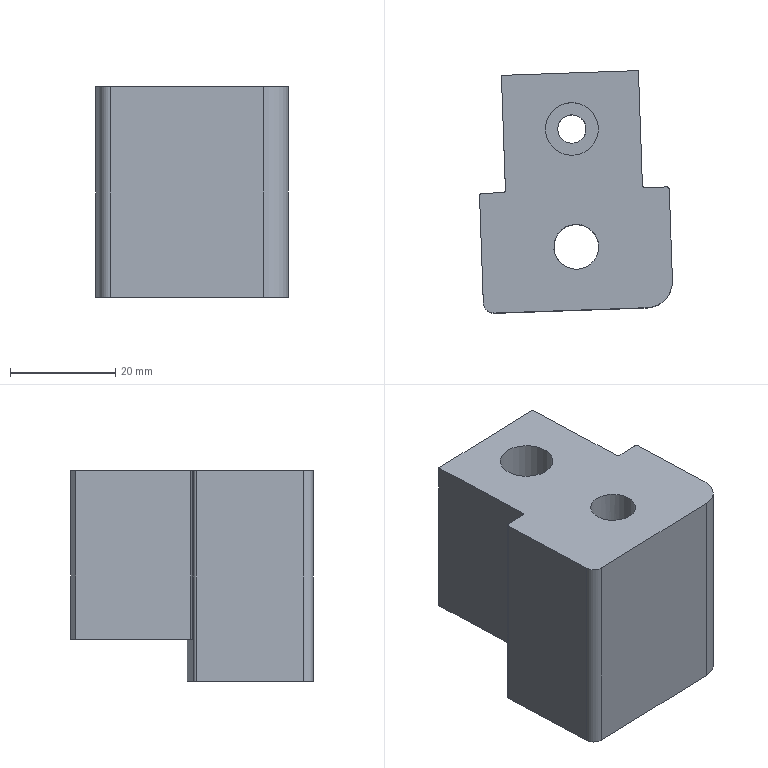Part | NX | features PS-24 2 | 1 solid | 22 faces | box 36.584 x 45.984 x 40 mm | volume 45410 mm3 | plane 12 | cylinder 10 | commonest cylinder face diameters 1 x4 10 x2 4 x1 5.4 x1 8.506 x1 14.5 x1
STEP:
#1=CARTESIAN_POINT('',(3172.903,-799.38,868.716));
#2=VERTEX_POINT('',#1);
#3=CARTESIAN_POINT('',(3198.887,-798.472,868.716));
#4=VERTEX_POINT('',#3);
#5=CARTESIAN_POINT('',(3185.895,-798.926,868.716));
#6=DIRECTION('',(0.9994,0.0349,0.));
#7=VECTOR('',#6,1000.);
#8=LINE('',#5,#7);
#9=EDGE_CURVE('',#2,#4,#8,.T.);
#10=ORIENTED_EDGE('',*,*,#9,.T.);
#11=CARTESIAN_POINT('',(3199.646,-820.196,868.716));
#12=VERTEX_POINT('',#11);
#13=CARTESIAN_POINT('',(3198.921,-799.44,868.716));
#14=DIRECTION('',(0.0349,-0.9994,0.));
#15=VECTOR('',#14,1000.);
#16=LINE('',#13,#15);
#17=EDGE_CURVE('',#4,#12,#16,.T.);
#18=ORIENTED_EDGE('',*,*,#17,.T.);
#19=CARTESIAN_POINT('',(3200.163,-820.678,868.716));
#20=VERTEX_POINT('',#19);
#21=CARTESIAN_POINT('',(3200.145,-820.179,868.716));
#22=DIRECTION('',(0.,0.,1.));
#23=DIRECTION('',(-1.,0.,0.));
#24=AXIS2_PLACEMENT_3D('',#21,#22,#23);
#25=CIRCLE('',#24,0.5);
#26=EDGE_CURVE('',#20,#12,#25,.F.);
#27=ORIENTED_EDGE('',*,*,#26,.F.);
#28=CARTESIAN_POINT('',(3173.179,-821.621,868.716));
#29=VERTEX_POINT('',#28);
#30=CARTESIAN_POINT('',(3186.671,-821.149,868.716));
#31=DIRECTION('',(0.9994,0.0349,0.));
#32=VECTOR('',#31,1000.);
#33=LINE('',#30,#32);
#34=EDGE_CURVE('',#29,#20,#33,.T.);
#35=ORIENTED_EDGE('',*,*,#34,.F.);
#36=CARTESIAN_POINT('',(3173.662,-821.103,868.716));
#37=VERTEX_POINT('',#36);
#38=CARTESIAN_POINT('',(3173.162,-821.121,868.716));
#39=DIRECTION('',(0.,0.,1.));
#40=DIRECTION('',(-1.,0.,0.));
#41=AXIS2_PLACEMENT_3D('',#38,#39,#40);
#42=CIRCLE('',#41,0.5);
#43=EDGE_CURVE('',#37,#29,#42,.F.);
#44=ORIENTED_EDGE('',*,*,#43,.F.);
#45=CARTESIAN_POINT('',(3172.937,-800.347,868.716));
#46=DIRECTION('',(-0.0349,0.9994,0.));
#47=VECTOR('',#46,1000.);
#48=LINE('',#45,#47);
#49=EDGE_CURVE('',#2,#37,#48,.F.);
#50=ORIENTED_EDGE('',*,*,#49,.F.);
#51=EDGE_LOOP('',(#10,#18,#27,#35,#44,#50));
#52=FACE_BOUND('',#51,.T.);
#53=CARTESIAN_POINT('',(3183.566,-809.538,868.716));
#54=VERTEX_POINT('',#53);
#55=CARTESIAN_POINT('',(3186.266,-809.538,868.716));
#56=DIRECTION('',(0.,0.,1.));
#57=DIRECTION('',(-1.,0.,0.));
#58=AXIS2_PLACEMENT_3D('',#55,#56,#57);
#59=CIRCLE('',#58,2.7);
#60=EDGE_CURVE('',#54,#54,#59,.F.);
#61=ORIENTED_EDGE('',*,*,#60,.F.);
#62=EDGE_LOOP('',(#61));
#63=FACE_BOUND('',#62,.T.);
#64=CARTESIAN_POINT('',(3186.266,-809.538,868.716));
#65=DIRECTION('',(0.,0.,-1.));
#66=DIRECTION('',(-0.0349,0.9994,0.));
#67=AXIS2_PLACEMENT_3D('',#64,#65,#66);
#68=PLANE('',#67);
#69=ADVANCED_FACE('',(#52,#63),#68,.T.);
#70=CARTESIAN_POINT('',(3186.266,-804.538,900.716));
#71=VERTEX_POINT('',#70);
#72=CARTESIAN_POINT('',(3186.266,-809.538,900.716));
#73=DIRECTION('',(0.,0.,-1.));
#74=DIRECTION('',(0.,1.,0.));
#75=AXIS2_PLACEMENT_3D('',#72,#73,#74);
#76=CIRCLE('',#75,5.);
#77=EDGE_CURVE('',#71,#71,#76,.T.);
#78=ORIENTED_EDGE('',*,*,#77,.T.);
#79=EDGE_LOOP('',(#78));
#80=FACE_BOUND('',#79,.T.);
#81=CARTESIAN_POINT('',(3172.903,-799.38,900.716));
#82=VERTEX_POINT('',#81);
#83=CARTESIAN_POINT('',(3173.662,-821.103,900.716));
#84=VERTEX_POINT('',#83);
#85=CARTESIAN_POINT('',(3172.937,-800.347,900.716));
#86=DIRECTION('',(0.0349,-0.9994,0.));
#87=VECTOR('',#86,1000.);
#88=LINE('',#85,#87);
#89=EDGE_CURVE('',#82,#84,#88,.T.);
#90=ORIENTED_EDGE('',*,*,#89,.T.);
#91=CARTESIAN_POINT('',(3173.179,-821.621,900.716));
#92=VERTEX_POINT('',#91);
#93=CARTESIAN_POINT('',(3173.162,-821.121,900.716));
#94=DIRECTION('',(0.,0.,-1.));
#95=DIRECTION('',(0.,1.,0.));
#96=AXIS2_PLACEMENT_3D('',#93,#94,#95);
#97=CIRCLE('',#96,0.5);
#98=EDGE_CURVE('',#92,#84,#97,.F.);
#99=ORIENTED_EDGE('',*,*,#98,.F.);
#100=CARTESIAN_POINT('',(3169.242,-821.758,900.716));
#101=VERTEX_POINT('',#100);
#102=CARTESIAN_POINT('',(3027.832,-826.696,900.716));
#103=DIRECTION('',(-0.9994,-0.0349,0.));
#104=VECTOR('',#103,1000.);
#105=LINE('',#102,#104);
#106=EDGE_CURVE('',#101,#92,#105,.F.);
#107=ORIENTED_EDGE('',*,*,#106,.F.);
#108=CARTESIAN_POINT('',(3168.76,-822.275,900.716));
#109=VERTEX_POINT('',#108);
#110=CARTESIAN_POINT('',(3169.26,-822.258,900.716));
#111=DIRECTION('',(0.,0.,-1.));
#112=DIRECTION('',(0.,1.,0.));
#113=AXIS2_PLACEMENT_3D('',#110,#111,#112);
#114=CIRCLE('',#113,0.5);
#115=EDGE_CURVE('',#109,#101,#114,.T.);
#116=ORIENTED_EDGE('',*,*,#115,.F.);
#117=CARTESIAN_POINT('',(3169.467,-842.526,900.716));
#118=VERTEX_POINT('',#117);
#119=CARTESIAN_POINT('',(3166.834,-767.126,900.716));
#120=DIRECTION('',(-0.0349,0.9994,0.));
#121=VECTOR('',#120,1000.);
#122=LINE('',#119,#121);
#123=EDGE_CURVE('',#109,#118,#122,.F.);
#124=ORIENTED_EDGE('',*,*,#123,.T.);
#125=CARTESIAN_POINT('',(3171.536,-844.455,900.716));
#126=VERTEX_POINT('',#125);
#127=CARTESIAN_POINT('',(3171.466,-842.456,900.716));
#128=DIRECTION('',(0.,0.,-1.));
#129=DIRECTION('',(0.,1.,0.));
#130=AXIS2_PLACEMENT_3D('',#127,#128,#129);
#131=CIRCLE('',#130,2.);
#132=EDGE_CURVE('',#118,#126,#131,.F.);
#133=ORIENTED_EDGE('',*,*,#132,.T.);
#134=CARTESIAN_POINT('',(3200.518,-843.443,900.716));
#135=VERTEX_POINT('',#134);
#136=CARTESIAN_POINT('',(3158.544,-844.908,900.716));
#137=DIRECTION('',(-0.9994,-0.0349,0.));
#138=VECTOR('',#137,1000.);
#139=LINE('',#136,#138);
#140=EDGE_CURVE('',#135,#126,#139,.T.);
#141=ORIENTED_EDGE('',*,*,#140,.F.);
#142=CARTESIAN_POINT('',(3205.34,-838.271,900.716));
#143=VERTEX_POINT('',#142);
#144=CARTESIAN_POINT('',(3200.343,-838.446,900.716));
#145=DIRECTION('',(0.,0.,-1.));
#146=DIRECTION('',(0.,1.,0.));
#147=AXIS2_PLACEMENT_3D('',#144,#145,#146);
#148=CIRCLE('',#147,5.);
#149=EDGE_CURVE('',#135,#143,#148,.F.);
#150=ORIENTED_EDGE('',*,*,#149,.T.);
#151=CARTESIAN_POINT('',(3204.738,-821.019,900.716));
#152=VERTEX_POINT('',#151);
#153=CARTESIAN_POINT('',(3202.812,-765.869,900.716));
#154=DIRECTION('',(-0.0349,0.9994,0.));
#155=VECTOR('',#154,1000.);
#156=LINE('',#153,#155);
#157=EDGE_CURVE('',#152,#143,#156,.F.);
#158=ORIENTED_EDGE('',*,*,#157,.F.);
#159=CARTESIAN_POINT('',(3204.221,-820.537,900.716));
#160=VERTEX_POINT('',#159);
#161=CARTESIAN_POINT('',(3204.238,-821.036,900.716));
#162=DIRECTION('',(0.,0.,-1.));
#163=DIRECTION('',(0.,1.,0.));
#164=AXIS2_PLACEMENT_3D('',#161,#162,#163);
#165=CIRCLE('',#164,0.5);
#166=EDGE_CURVE('',#160,#152,#165,.T.);
#167=ORIENTED_EDGE('',*,*,#166,.F.);
#168=CARTESIAN_POINT('',(3200.163,-820.678,900.716));
#169=VERTEX_POINT('',#168);
#170=CARTESIAN_POINT('',(3027.832,-826.696,900.716));
#171=DIRECTION('',(-0.9994,-0.0349,0.));
#172=VECTOR('',#171,1000.);
#173=LINE('',#170,#172);
#174=EDGE_CURVE('',#169,#160,#173,.F.);
#175=ORIENTED_EDGE('',*,*,#174,.F.);
#176=CARTESIAN_POINT('',(3199.646,-820.196,900.716));
#177=VERTEX_POINT('',#176);
#178=CARTESIAN_POINT('',(3200.145,-820.179,900.716));
#179=DIRECTION('',(0.,0.,-1.));
#180=DIRECTION('',(0.,1.,0.));
#181=AXIS2_PLACEMENT_3D('',#178,#179,#180);
#182=CIRCLE('',#181,0.5);
#183=EDGE_CURVE('',#177,#169,#182,.F.);
#184=ORIENTED_EDGE('',*,*,#183,.F.);
#185=CARTESIAN_POINT('',(3198.887,-798.472,900.716));
#186=VERTEX_POINT('',#185);
#187=CARTESIAN_POINT('',(3198.921,-799.44,900.716));
#188=DIRECTION('',(-0.0349,0.9994,0.));
#189=VECTOR('',#188,1000.);
#190=LINE('',#187,#189);
#191=EDGE_CURVE('',#186,#177,#190,.F.);
#192=ORIENTED_EDGE('',*,*,#191,.F.);
#193=CARTESIAN_POINT('',(3027.056,-804.472,900.716));
#194=DIRECTION('',(-0.9994,-0.0349,0.));
#195=VECTOR('',#194,1000.);
#196=LINE('',#193,#195);
#197=EDGE_CURVE('',#82,#186,#196,.F.);
#198=ORIENTED_EDGE('',*,*,#197,.F.);
#199=EDGE_LOOP('',(#90,#99,#107,#116,#124,#133,#141,#150,#158,#167,#175,#184,#192,#198));
#200=FACE_BOUND('',#199,.T.);
#201=CARTESIAN_POINT('',(3187.107,-827.651,900.716));
#202=VERTEX_POINT('',#201);
#203=CARTESIAN_POINT('',(3187.107,-831.904,900.716));
#204=DIRECTION('',(0.,0.,-1.));
#205=DIRECTION('',(0.,1.,0.));
#206=AXIS2_PLACEMENT_3D('',#203,#204,#205);
#207=CIRCLE('',#206,4.253);
#208=EDGE_CURVE('',#202,#202,#207,.T.);
#209=ORIENTED_EDGE('',*,*,#208,.T.);
#210=EDGE_LOOP('',(#209));
#211=FACE_BOUND('',#210,.T.);
#212=CARTESIAN_POINT('',(3025.924,-772.046,900.716));
#213=DIRECTION('',(0.,0.,1.));
#214=DIRECTION('',(0.9976,0.06975,0.));
#215=AXIS2_PLACEMENT_3D('',#212,#213,#214);
#216=PLANE('',#215);
#217=ADVANCED_FACE('',(#80,#200,#211),#216,.T.);
#218=ORIENTED_EDGE('',*,*,#17,.F.);
#219=CARTESIAN_POINT('',(3198.887,-798.472,880.716));
#220=DIRECTION('',(0.,0.,-1.));
#221=VECTOR('',#220,1000.);
#222=LINE('',#219,#221);
#223=EDGE_CURVE('',#186,#4,#222,.T.);
#224=ORIENTED_EDGE('',*,*,#223,.F.);
#225=ORIENTED_EDGE('',*,*,#191,.T.);
#226=CARTESIAN_POINT('',(3199.646,-820.196,830.716));
#227=DIRECTION('',(0.,0.,1.));
#228=VECTOR('',#227,1000.);
#229=LINE('',#226,#228);
#230=EDGE_CURVE('',#12,#177,#229,.T.);
#231=ORIENTED_EDGE('',*,*,#230,.F.);
#232=EDGE_LOOP('',(#218,#224,#225,#231));
#233=FACE_BOUND('',#232,.T.);
#234=CARTESIAN_POINT('',(3198.921,-799.44,830.716));
#235=DIRECTION('',(0.9994,0.0349,0.));
#236=DIRECTION('',(0.0349,-0.9994,0.));
#237=AXIS2_PLACEMENT_3D('',#234,#235,#236);
#238=PLANE('',#237);
#239=ADVANCED_FACE('',(#233),#238,.T.);
#240=ORIENTED_EDGE('',*,*,#49,.T.);
#241=CARTESIAN_POINT('',(3173.662,-821.103,863.216));
#242=DIRECTION('',(0.,0.,1.));
#243=VECTOR('',#242,1000.);
#244=LINE('',#241,#243);
#245=EDGE_CURVE('',#84,#37,#244,.F.);
#246=ORIENTED_EDGE('',*,*,#245,.F.);
#247=ORIENTED_EDGE('',*,*,#89,.F.);
#248=CARTESIAN_POINT('',(3172.903,-799.38,830.716));
#249=DIRECTION('',(0.,0.,-1.));
#250=VECTOR('',#249,1000.);
#251=LINE('',#248,#250);
#252=EDGE_CURVE('',#82,#2,#251,.T.);
#253=ORIENTED_EDGE('',*,*,#252,.T.);
#254=EDGE_LOOP('',(#240,#246,#247,#253));
#255=FACE_BOUND('',#254,.T.);
#256=CARTESIAN_POINT('',(3172.937,-800.347,830.716));
#257=DIRECTION('',(-0.9994,-0.0349,0.));
#258=DIRECTION('',(-0.0349,0.9994,0.));
#259=AXIS2_PLACEMENT_3D('',#256,#257,#258);
#260=PLANE('',#259);
#261=ADVANCED_FACE('',(#255),#260,.T.);
#262=CARTESIAN_POINT('',(3186.266,-814.538,890.716));
#263=VERTEX_POINT('',#262);
#264=CARTESIAN_POINT('',(3186.266,-809.538,890.716));
#265=DIRECTION('',(0.,0.,1.));
#266=DIRECTION('',(0.,-1.,0.));
#267=AXIS2_PLACEMENT_3D('',#264,#265,#266);
#268=CIRCLE('',#267,5.);
#269=EDGE_CURVE('',#263,#263,#268,.F.);
#270=ORIENTED_EDGE('',*,*,#269,.T.);
#271=EDGE_LOOP('',(#270));
#272=FACE_BOUND('',#271,.T.);
#273=ORIENTED_EDGE('',*,*,#77,.F.);
#274=EDGE_LOOP('',(#273));
#275=FACE_BOUND('',#274,.T.);
#276=CARTESIAN_POINT('',(3186.266,-809.538,935.716));
#277=DIRECTION('',(0.,0.,-1.));
#278=DIRECTION('',(0.9976,0.06975,0.));
#279=AXIS2_PLACEMENT_3D('',#276,#277,#278);
#280=CYLINDRICAL_SURFACE('',#279,5.);
#281=ADVANCED_FACE('',(#272,#275),#280,.F.);
#282=ORIENTED_EDGE('',*,*,#60,.T.);
#283=EDGE_LOOP('',(#282));
#284=FACE_BOUND('',#283,.T.);
#285=CARTESIAN_POINT('',(3186.266,-812.238,890.716));
#286=VERTEX_POINT('',#285);
#287=CARTESIAN_POINT('',(3186.266,-809.538,890.716));
#288=DIRECTION('',(0.,0.,1.));
#289=DIRECTION('',(0.,-1.,0.));
#290=AXIS2_PLACEMENT_3D('',#287,#288,#289);
#291=CIRCLE('',#290,2.7);
#292=EDGE_CURVE('',#286,#286,#291,.T.);
#293=ORIENTED_EDGE('',*,*,#292,.T.);
#294=EDGE_LOOP('',(#293));
#295=FACE_BOUND('',#294,.T.);
#296=CARTESIAN_POINT('',(3186.266,-809.538,872.716));
#297=DIRECTION('',(0.,0.,-1.));
#298=DIRECTION('',(0.9976,0.06975,0.));
#299=AXIS2_PLACEMENT_3D('',#296,#297,#298);
#300=CYLINDRICAL_SURFACE('',#299,2.7);
#301=ADVANCED_FACE('',(#284,#295),#300,.F.);
#302=ORIENTED_EDGE('',*,*,#292,.F.);
#303=EDGE_LOOP('',(#302));
#304=FACE_BOUND('',#303,.T.);
#305=ORIENTED_EDGE('',*,*,#269,.F.);
#306=EDGE_LOOP('',(#305));
#307=FACE_BOUND('',#306,.T.);
#308=CARTESIAN_POINT('',(3186.266,-809.538,890.716));
#309=DIRECTION('',(0.,0.,-1.));
#310=DIRECTION('',(-0.9976,-0.06975,0.));
#311=AXIS2_PLACEMENT_3D('',#308,#309,#310);
#312=PLANE('',#311);
#313=ADVANCED_FACE('',(#304,#307),#312,.F.);
#314=ORIENTED_EDGE('',*,*,#183,.T.);
#315=CARTESIAN_POINT('',(3200.163,-820.678,863.216));
#316=DIRECTION('',(0.,0.,1.));
#317=VECTOR('',#316,1000.);
#318=LINE('',#315,#317);
#319=EDGE_CURVE('',#169,#20,#318,.F.);
#320=ORIENTED_EDGE('',*,*,#319,.T.);
#321=ORIENTED_EDGE('',*,*,#26,.T.);
#322=ORIENTED_EDGE('',*,*,#230,.T.);
#323=EDGE_LOOP('',(#314,#320,#321,#322));
#324=FACE_BOUND('',#323,.T.);
#325=CARTESIAN_POINT('',(3200.145,-820.179,830.716));
#326=DIRECTION('',(0.,0.,1.));
#327=DIRECTION('',(0.,1.,0.));
#328=AXIS2_PLACEMENT_3D('',#325,#326,#327);
#329=CYLINDRICAL_SURFACE('',#328,0.5);
#330=ADVANCED_FACE('',(#324),#329,.F.);
#331=ORIENTED_EDGE('',*,*,#98,.T.);
#332=ORIENTED_EDGE('',*,*,#245,.T.);
#333=ORIENTED_EDGE('',*,*,#43,.T.);
#334=CARTESIAN_POINT('',(3173.179,-821.621,863.216));
#335=DIRECTION('',(0.,0.,-1.));
#336=VECTOR('',#335,1000.);
#337=LINE('',#334,#336);
#338=EDGE_CURVE('',#29,#92,#337,.F.);
#339=ORIENTED_EDGE('',*,*,#338,.T.);
#340=EDGE_LOOP('',(#331,#332,#333,#339));
#341=FACE_BOUND('',#340,.T.);
#342=CARTESIAN_POINT('',(3173.162,-821.121,863.216));
#343=DIRECTION('',(0.,0.,1.));
#344=DIRECTION('',(0.,1.,0.));
#345=AXIS2_PLACEMENT_3D('',#342,#343,#344);
#346=CYLINDRICAL_SURFACE('',#345,0.5);
#347=ADVANCED_FACE('',(#341),#346,.F.);
#348=ORIENTED_EDGE('',*,*,#34,.T.);
#349=ORIENTED_EDGE('',*,*,#319,.F.);
#350=ORIENTED_EDGE('',*,*,#174,.T.);
#351=CARTESIAN_POINT('',(3204.221,-820.537,860.716));
#352=VERTEX_POINT('',#351);
#353=CARTESIAN_POINT('',(3204.221,-820.537,890.716));
#354=DIRECTION('',(0.,0.,1.));
#355=VECTOR('',#354,1000.);
#356=LINE('',#353,#355);
#357=EDGE_CURVE('',#352,#160,#356,.T.);
#358=ORIENTED_EDGE('',*,*,#357,.F.);
#359=CARTESIAN_POINT('',(3169.242,-821.758,860.716));
#360=VERTEX_POINT('',#359);
#361=CARTESIAN_POINT('',(2864.273,-832.407,860.716));
#362=DIRECTION('',(0.9994,0.0349,0.));
#363=VECTOR('',#362,1000.);
#364=LINE('',#361,#363);
#365=EDGE_CURVE('',#352,#360,#364,.F.);
#366=ORIENTED_EDGE('',*,*,#365,.T.);
#367=CARTESIAN_POINT('',(3169.242,-821.758,863.216));
#368=DIRECTION('',(0.,0.,1.));
#369=VECTOR('',#368,1000.);
#370=LINE('',#367,#369);
#371=EDGE_CURVE('',#101,#360,#370,.F.);
#372=ORIENTED_EDGE('',*,*,#371,.F.);
#373=ORIENTED_EDGE('',*,*,#106,.T.);
#374=ORIENTED_EDGE('',*,*,#338,.F.);
#375=EDGE_LOOP('',(#348,#349,#350,#358,#366,#372,#373,#374));
#376=FACE_BOUND('',#375,.T.);
#377=CARTESIAN_POINT('',(3183.542,-821.259,863.216));
#378=DIRECTION('',(0.0349,-0.9994,0.));
#379=DIRECTION('',(-0.9994,-0.0349,0.));
#380=AXIS2_PLACEMENT_3D('',#377,#378,#379);
#381=PLANE('',#380);
#382=ADVANCED_FACE('',(#376),#381,.F.);
#383=CARTESIAN_POINT('',(3191.35,-831.607,879.716));
#384=VERTEX_POINT('',#383);
#385=CARTESIAN_POINT('',(3187.107,-831.904,879.716));
#386=DIRECTION('',(0.,0.,1.));
#387=DIRECTION('',(0.9976,0.06975,0.));
#388=AXIS2_PLACEMENT_3D('',#385,#386,#387);
#389=CIRCLE('',#388,4.253);
#390=EDGE_CURVE('',#384,#384,#389,.T.);
#391=ORIENTED_EDGE('',*,*,#390,.T.);
#392=EDGE_LOOP('',(#391));
#393=FACE_BOUND('',#392,.T.);
#394=CARTESIAN_POINT('',(3194.339,-831.398,879.716));
#395=VERTEX_POINT('',#394);
#396=CARTESIAN_POINT('',(3187.107,-831.904,879.716));
#397=DIRECTION('',(0.,0.,-1.));
#398=DIRECTION('',(0.9976,0.06975,0.));
#399=AXIS2_PLACEMENT_3D('',#396,#397,#398);
#400=CIRCLE('',#399,7.25);
#401=EDGE_CURVE('',#395,#395,#400,.F.);
#402=ORIENTED_EDGE('',*,*,#401,.F.);
#403=EDGE_LOOP('',(#402));
#404=FACE_BOUND('',#403,.T.);
#405=CARTESIAN_POINT('',(3187.107,-831.904,879.716));
#406=DIRECTION('',(0.,0.,1.));
#407=DIRECTION('',(0.9976,0.06975,0.));
#408=AXIS2_PLACEMENT_3D('',#405,#406,#407);
#409=PLANE('',#408);
#410=ADVANCED_FACE('',(#393,#404),#409,.F.);
#411=ORIENTED_EDGE('',*,*,#390,.F.);
#412=EDGE_LOOP('',(#411));
#413=FACE_BOUND('',#412,.T.);
#414=ORIENTED_EDGE('',*,*,#208,.F.);
#415=EDGE_LOOP('',(#414));
#416=FACE_BOUND('',#415,.T.);
#417=CARTESIAN_POINT('',(3187.107,-831.904,868.716));
#418=DIRECTION('',(0.,0.,1.));
#419=DIRECTION('',(0.9976,0.06975,0.));
#420=AXIS2_PLACEMENT_3D('',#417,#418,#419);
#421=CYLINDRICAL_SURFACE('',#420,4.253);
#422=ADVANCED_FACE('',(#413,#416),#421,.F.);
#423=CARTESIAN_POINT('',(3168.76,-822.275,860.716));
#424=VERTEX_POINT('',#423);
#425=CARTESIAN_POINT('',(3169.26,-822.258,860.716));
#426=DIRECTION('',(0.,0.,1.));
#427=DIRECTION('',(1.,0.,0.));
#428=AXIS2_PLACEMENT_3D('',#425,#426,#427);
#429=CIRCLE('',#428,0.5);
#430=EDGE_CURVE('',#360,#424,#429,.T.);
#431=ORIENTED_EDGE('',*,*,#430,.T.);
#432=CARTESIAN_POINT('',(3168.76,-822.275,890.716));
#433=DIRECTION('',(0.,0.,1.));
#434=VECTOR('',#433,1000.);
#435=LINE('',#432,#434);
#436=EDGE_CURVE('',#424,#109,#435,.T.);
#437=ORIENTED_EDGE('',*,*,#436,.T.);
#438=ORIENTED_EDGE('',*,*,#115,.T.);
#439=ORIENTED_EDGE('',*,*,#371,.T.);
#440=EDGE_LOOP('',(#431,#437,#438,#439));
#441=FACE_BOUND('',#440,.T.);
#442=CARTESIAN_POINT('',(3169.26,-822.258,890.716));
#443=DIRECTION('',(0.,0.,1.));
#444=DIRECTION('',(1.,0.,0.));
#445=AXIS2_PLACEMENT_3D('',#442,#443,#444);
#446=CYLINDRICAL_SURFACE('',#445,0.5);
#447=ADVANCED_FACE('',(#441),#446,.T.);
#448=CARTESIAN_POINT('',(3169.467,-842.526,860.716));
#449=VERTEX_POINT('',#448);
#450=CARTESIAN_POINT('',(3174.564,-988.491,860.716));
#451=DIRECTION('',(-0.0349,0.9994,0.));
#452=VECTOR('',#451,1000.);
#453=LINE('',#450,#452);
#454=EDGE_CURVE('',#424,#449,#453,.F.);
#455=ORIENTED_EDGE('',*,*,#454,.T.);
#456=CARTESIAN_POINT('',(3169.467,-842.526,890.716));
#457=DIRECTION('',(0.,0.,1.));
#458=VECTOR('',#457,1000.);
#459=LINE('',#456,#458);
#460=EDGE_CURVE('',#449,#118,#459,.T.);
#461=ORIENTED_EDGE('',*,*,#460,.T.);
#462=ORIENTED_EDGE('',*,*,#123,.F.);
#463=ORIENTED_EDGE('',*,*,#436,.F.);
#464=EDGE_LOOP('',(#455,#461,#462,#463));
#465=FACE_BOUND('',#464,.T.);
#466=CARTESIAN_POINT('',(3168.523,-815.501,890.716));
#467=DIRECTION('',(0.9994,0.0349,0.));
#468=DIRECTION('',(-0.0349,0.9994,0.));
#469=AXIS2_PLACEMENT_3D('',#466,#467,#468);
#470=PLANE('',#469);
#471=ADVANCED_FACE('',(#465),#470,.F.);
#472=ORIENTED_EDGE('',*,*,#132,.F.);
#473=ORIENTED_EDGE('',*,*,#460,.F.);
#474=CARTESIAN_POINT('',(3171.536,-844.455,860.716));
#475=VERTEX_POINT('',#474);
#476=CARTESIAN_POINT('',(3171.466,-842.456,860.716));
#477=DIRECTION('',(0.,0.,1.));
#478=DIRECTION('',(1.,0.,0.));
#479=AXIS2_PLACEMENT_3D('',#476,#477,#478);
#480=CIRCLE('',#479,2.);
#481=EDGE_CURVE('',#475,#449,#480,.F.);
#482=ORIENTED_EDGE('',*,*,#481,.F.);
#483=CARTESIAN_POINT('',(3171.536,-844.455,860.716));
#484=DIRECTION('',(0.,0.,-1.));
#485=VECTOR('',#484,1000.);
#486=LINE('',#483,#485);
#487=EDGE_CURVE('',#126,#475,#486,.T.);
#488=ORIENTED_EDGE('',*,*,#487,.F.);
#489=EDGE_LOOP('',(#472,#473,#482,#488));
#490=FACE_BOUND('',#489,.T.);
#491=CARTESIAN_POINT('',(3171.466,-842.456,935.716));
#492=DIRECTION('',(0.,0.,-1.));
#493=DIRECTION('',(-0.9976,-0.06975,0.));
#494=AXIS2_PLACEMENT_3D('',#491,#492,#493);
#495=CYLINDRICAL_SURFACE('',#494,2.);
#496=ADVANCED_FACE('',(#490),#495,.T.);
#497=CARTESIAN_POINT('',(3200.518,-843.443,860.716));
#498=VERTEX_POINT('',#497);
#499=CARTESIAN_POINT('',(3158.544,-844.908,860.716));
#500=DIRECTION('',(0.9994,0.0349,0.));
#501=VECTOR('',#500,1000.);
#502=LINE('',#499,#501);
#503=EDGE_CURVE('',#475,#498,#502,.T.);
#504=ORIENTED_EDGE('',*,*,#503,.T.);
#505=CARTESIAN_POINT('',(3200.518,-843.443,935.716));
#506=DIRECTION('',(0.,0.,-1.));
#507=VECTOR('',#506,1000.);
#508=LINE('',#505,#507);
#509=EDGE_CURVE('',#498,#135,#508,.F.);
#510=ORIENTED_EDGE('',*,*,#509,.T.);
#511=ORIENTED_EDGE('',*,*,#140,.T.);
#512=ORIENTED_EDGE('',*,*,#487,.T.);
#513=EDGE_LOOP('',(#504,#510,#511,#512));
#514=FACE_BOUND('',#513,.T.);
#515=CARTESIAN_POINT('',(3158.544,-844.908,935.716));
#516=DIRECTION('',(-0.0349,0.9994,0.));
#517=DIRECTION('',(-0.9994,-0.0349,0.));
#518=AXIS2_PLACEMENT_3D('',#515,#516,#517);
#519=PLANE('',#518);
#520=ADVANCED_FACE('',(#514),#519,.F.);
#521=ORIENTED_EDGE('',*,*,#149,.F.);
#522=ORIENTED_EDGE('',*,*,#509,.F.);
#523=CARTESIAN_POINT('',(3205.34,-838.271,860.716));
#524=VERTEX_POINT('',#523);
#525=CARTESIAN_POINT('',(3200.343,-838.446,860.716));
#526=DIRECTION('',(0.,0.,1.));
#527=DIRECTION('',(1.,0.,0.));
#528=AXIS2_PLACEMENT_3D('',#525,#526,#527);
#529=CIRCLE('',#528,5.);
#530=EDGE_CURVE('',#524,#498,#529,.F.);
#531=ORIENTED_EDGE('',*,*,#530,.F.);
#532=CARTESIAN_POINT('',(3205.34,-838.271,862.716));
#533=DIRECTION('',(0.,0.,1.));
#534=VECTOR('',#533,1000.);
#535=LINE('',#532,#534);
#536=EDGE_CURVE('',#143,#524,#535,.F.);
#537=ORIENTED_EDGE('',*,*,#536,.F.);
#538=EDGE_LOOP('',(#521,#522,#531,#537));
#539=FACE_BOUND('',#538,.T.);
#540=CARTESIAN_POINT('',(3200.343,-838.446,862.716));
#541=DIRECTION('',(0.,0.,1.));
#542=DIRECTION('',(0.9976,0.06975,0.));
#543=AXIS2_PLACEMENT_3D('',#540,#541,#542);
#544=CYLINDRICAL_SURFACE('',#543,5.);
#545=ADVANCED_FACE('',(#539),#544,.T.);
#546=ORIENTED_EDGE('',*,*,#157,.T.);
#547=ORIENTED_EDGE('',*,*,#536,.T.);
#548=CARTESIAN_POINT('',(3204.738,-821.019,860.716));
#549=VERTEX_POINT('',#548);
#550=CARTESIAN_POINT('',(3210.542,-987.235,860.716));
#551=DIRECTION('',(-0.0349,0.9994,0.));
#552=VECTOR('',#551,1000.);
#553=LINE('',#550,#552);
#554=EDGE_CURVE('',#549,#524,#553,.F.);
#555=ORIENTED_EDGE('',*,*,#554,.F.);
#556=CARTESIAN_POINT('',(3204.738,-821.019,868.716));
#557=DIRECTION('',(0.,0.,1.));
#558=VECTOR('',#557,1000.);
#559=LINE('',#556,#558);
#560=EDGE_CURVE('',#152,#549,#559,.F.);
#561=ORIENTED_EDGE('',*,*,#560,.F.);
#562=EDGE_LOOP('',(#546,#547,#555,#561));
#563=FACE_BOUND('',#562,.T.);
#564=CARTESIAN_POINT('',(3204.536,-815.244,862.716));
#565=DIRECTION('',(0.9994,0.0349,0.));
#566=DIRECTION('',(-0.0349,0.9994,0.));
#567=AXIS2_PLACEMENT_3D('',#564,#565,#566);
#568=PLANE('',#567);
#569=ADVANCED_FACE('',(#563),#568,.T.);
#570=CARTESIAN_POINT('',(3204.238,-821.036,860.716));
#571=DIRECTION('',(0.,0.,1.));
#572=DIRECTION('',(1.,0.,0.));
#573=AXIS2_PLACEMENT_3D('',#570,#571,#572);
#574=CIRCLE('',#573,0.5);
#575=EDGE_CURVE('',#549,#352,#574,.T.);
#576=ORIENTED_EDGE('',*,*,#575,.T.);
#577=ORIENTED_EDGE('',*,*,#357,.T.);
#578=ORIENTED_EDGE('',*,*,#166,.T.);
#579=ORIENTED_EDGE('',*,*,#560,.T.);
#580=EDGE_LOOP('',(#576,#577,#578,#579));
#581=FACE_BOUND('',#580,.T.);
#582=CARTESIAN_POINT('',(3204.238,-821.036,863.216));
#583=DIRECTION('',(0.,0.,-1.));
#584=DIRECTION('',(-1.,0.,0.));
#585=AXIS2_PLACEMENT_3D('',#582,#583,#584);
#586=CYLINDRICAL_SURFACE('',#585,0.5);
#587=ADVANCED_FACE('',(#581),#586,.T.);
#588=ORIENTED_EDGE('',*,*,#401,.T.);
#589=EDGE_LOOP('',(#588));
#590=FACE_BOUND('',#589,.T.);
#591=CARTESIAN_POINT('',(3194.357,-831.904,860.716));
#592=VERTEX_POINT('',#591);
#593=CARTESIAN_POINT('',(3187.107,-831.904,860.716));
#594=DIRECTION('',(0.,0.,1.));
#595=DIRECTION('',(1.,0.,0.));
#596=AXIS2_PLACEMENT_3D('',#593,#594,#595);
#597=CIRCLE('',#596,7.25);
#598=EDGE_CURVE('',#592,#592,#597,.T.);
#599=ORIENTED_EDGE('',*,*,#598,.F.);
#600=EDGE_LOOP('',(#599));
#601=FACE_BOUND('',#600,.T.);
#602=CARTESIAN_POINT('',(3187.107,-831.904,868.716));
#603=DIRECTION('',(0.,0.,1.));
#604=DIRECTION('',(0.9976,0.06975,0.));
#605=AXIS2_PLACEMENT_3D('',#602,#603,#604);
#606=CYLINDRICAL_SURFACE('',#605,7.25);
#607=ADVANCED_FACE('',(#590,#601),#606,.F.);
#608=ORIENTED_EDGE('',*,*,#598,.T.);
#609=EDGE_LOOP('',(#608));
#610=FACE_BOUND('',#609,.T.);
#611=ORIENTED_EDGE('',*,*,#430,.F.);
#612=ORIENTED_EDGE('',*,*,#365,.F.);
#613=ORIENTED_EDGE('',*,*,#575,.F.);
#614=ORIENTED_EDGE('',*,*,#554,.T.);
#615=ORIENTED_EDGE('',*,*,#530,.T.);
#616=ORIENTED_EDGE('',*,*,#503,.F.);
#617=ORIENTED_EDGE('',*,*,#481,.T.);
#618=ORIENTED_EDGE('',*,*,#454,.F.);
#619=EDGE_LOOP('',(#611,#612,#613,#614,#615,#616,#617,#618));
#620=FACE_BOUND('',#619,.T.);
#621=CARTESIAN_POINT('',(2870.094,-999.122,860.716));
#622=DIRECTION('',(0.,0.,1.));
#623=DIRECTION('',(0.,1.,0.));
#624=AXIS2_PLACEMENT_3D('',#621,#622,#623);
#625=PLANE('',#624);
#626=ADVANCED_FACE('',(#610,#620),#625,.F.);
#627=ORIENTED_EDGE('',*,*,#9,.F.);
#628=ORIENTED_EDGE('',*,*,#252,.F.);
#629=ORIENTED_EDGE('',*,*,#197,.T.);
#630=ORIENTED_EDGE('',*,*,#223,.T.);
#631=EDGE_LOOP('',(#627,#628,#629,#630));
#632=FACE_BOUND('',#631,.T.);
#633=CARTESIAN_POINT('',(3183.957,-798.994,880.716));
#634=DIRECTION('',(0.0349,-0.9994,0.));
#635=DIRECTION('',(-0.9994,-0.0349,0.));
#636=AXIS2_PLACEMENT_3D('',#633,#634,#635);
#637=PLANE('',#636);
#638=ADVANCED_FACE('',(#632),#637,.F.);
#639=CLOSED_SHELL('',(#69,#217,#239,#261,#281,#301,#313,#330,#347,#382,#410,#422,#447,#471,#496,#520,#545,#569,#587,#607,#626,#638));
#640=MANIFOLD_SOLID_BREP('',#639);
#641=(LENGTH_UNIT()NAMED_UNIT(*)SI_UNIT(.MILLI.,.METRE.));
#642=UNCERTAINTY_MEASURE_WITH_UNIT(LENGTH_MEASURE(0.00001),#641,'','');
#643=(NAMED_UNIT(*)PLANE_ANGLE_UNIT()SI_UNIT($,.RADIAN.));
#644=(NAMED_UNIT(*)SI_UNIT($,.STERADIAN.)SOLID_ANGLE_UNIT());
#645=(GEOMETRIC_REPRESENTATION_CONTEXT(3)GLOBAL_UNCERTAINTY_ASSIGNED_CONTEXT((#642))GLOBAL_UNIT_ASSIGNED_CONTEXT((#641,#643,#644))REPRESENTATION_CONTEXT('',''));
#646=ADVANCED_BREP_SHAPE_REPRESENTATION('',(#640),#645);